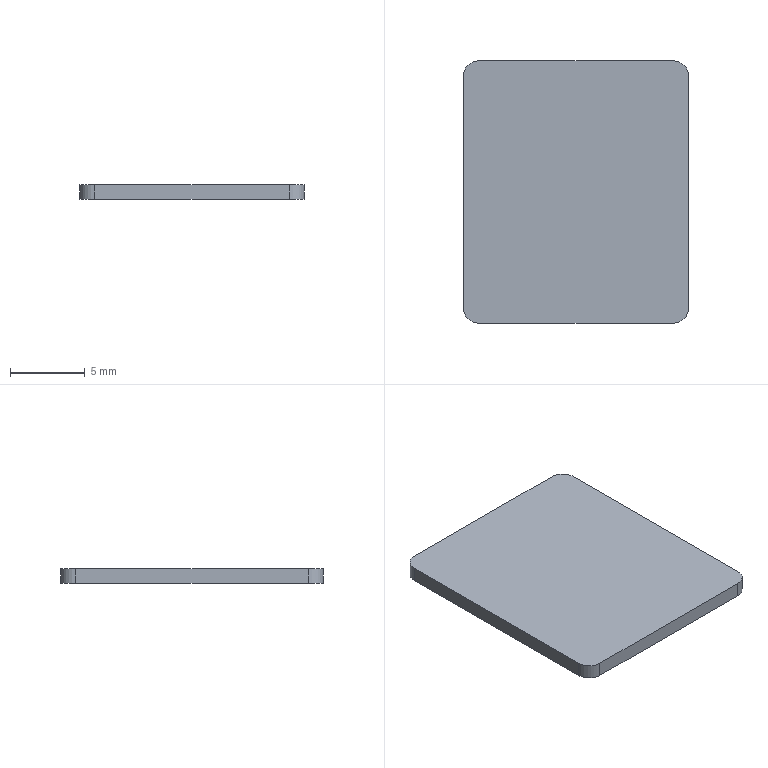Part | STEP file | 1 solid | 10 faces | box 15 x 17.5 x 1 mm | volume 261.642 mm3 | plane 6 | cylinder 4 | commonest cylinder face diameters 2 x4
STEP:
#1=CARTESIAN_POINT('',(0.,0.,0.));
#2=DIRECTION('',(0.,0.,1.));
#3=DIRECTION('',(1.,0.,0.));
#4=AXIS2_PLACEMENT_3D('',#1,#2,#3);
#5=CARTESIAN_POINT('',(6.5,6.5,38.7));
#6=VERTEX_POINT('',#5);
#7=CARTESIAN_POINT('',(-6.5,6.5,38.7));
#8=VERTEX_POINT('',#7);
#9=CARTESIAN_POINT('',(-6.5,6.5,38.7));
#10=DIRECTION('',(-1.,0.,0.));
#11=VECTOR('',#10,1.);
#12=LINE('',#9,#11);
#13=CARTESIAN_POINT('',(-6.5,5.5,38.7));
#14=DIRECTION('',(0.,0.,1.));
#15=DIRECTION('',(1.,0.,0.));
#16=AXIS2_PLACEMENT_3D('',#13,#14,#15);
#17=PLANE('',#16);
#18=CARTESIAN_POINT('',(0.,1.));
#19=DIRECTION('',(-1.,0.));
#20=VECTOR('',#19,1.);
#21=LINE('',#18,#20);
#22=(GEOMETRIC_REPRESENTATION_CONTEXT(2)PARAMETRIC_REPRESENTATION_CONTEXT()REPRESENTATION_CONTEXT('',''));
#23=DEFINITIONAL_REPRESENTATION('',(#21),#22);
#24=PCURVE('',#17,#23);
#25=CARTESIAN_POINT('',(6.5,6.5,39.7));
#26=DIRECTION('',(0.,-1.,0.));
#27=DIRECTION('',(0.,0.,-1.));
#28=AXIS2_PLACEMENT_3D('',#25,#26,#27);
#29=PLANE('',#28);
#30=CARTESIAN_POINT('',(1.,-13.));
#31=DIRECTION('',(0.,-1.));
#32=VECTOR('',#31,1.);
#33=LINE('',#30,#32);
#34=(GEOMETRIC_REPRESENTATION_CONTEXT(2)PARAMETRIC_REPRESENTATION_CONTEXT()REPRESENTATION_CONTEXT('',''));
#35=DEFINITIONAL_REPRESENTATION('',(#33),#34);
#36=PCURVE('',#29,#35);
#37=SURFACE_CURVE('',#12,(#24,#36),.PCURVE_S1.);
#38=EDGE_CURVE('',#6,#8,#37,.T.);
#39=ORIENTED_EDGE('',*,*,#38,.F.);
#40=CARTESIAN_POINT('',(7.5,5.5,38.7));
#41=VERTEX_POINT('',#40);
#42=CARTESIAN_POINT('',(6.5,5.5,38.7));
#43=DIRECTION('',(0.,0.,1.));
#44=DIRECTION('',(1.,0.,0.));
#45=AXIS2_PLACEMENT_3D('',#42,#43,#44);
#46=CIRCLE('',#45,1.);
#47=CARTESIAN_POINT('',(13.,0.));
#48=DIRECTION('',(1.,0.));
#49=AXIS2_PLACEMENT_2D('',#47,#48);
#50=CIRCLE('',#49,1.);
#51=(GEOMETRIC_REPRESENTATION_CONTEXT(2)PARAMETRIC_REPRESENTATION_CONTEXT()REPRESENTATION_CONTEXT('',''));
#52=DEFINITIONAL_REPRESENTATION('',(#50),#51);
#53=PCURVE('',#17,#52);
#54=CARTESIAN_POINT('',(6.5,5.5,39.7));
#55=DIRECTION('',(0.,0.,1.));
#56=DIRECTION('',(1.,0.,0.));
#57=AXIS2_PLACEMENT_3D('',#54,#55,#56);
#58=CYLINDRICAL_SURFACE('',#57,1.);
#59=CARTESIAN_POINT('',(0.,-1.));
#60=DIRECTION('',(1.,0.));
#61=VECTOR('',#60,1.);
#62=LINE('',#59,#61);
#63=(GEOMETRIC_REPRESENTATION_CONTEXT(2)PARAMETRIC_REPRESENTATION_CONTEXT()REPRESENTATION_CONTEXT('',''));
#64=DEFINITIONAL_REPRESENTATION('',(#62),#63);
#65=PCURVE('',#58,#64);
#66=SURFACE_CURVE('',#46,(#53,#65),.PCURVE_S1.);
#67=EDGE_CURVE('',#41,#6,#66,.T.);
#68=ORIENTED_EDGE('',*,*,#67,.F.);
#69=CARTESIAN_POINT('',(7.5,-10.,38.7));
#70=VERTEX_POINT('',#69);
#71=CARTESIAN_POINT('',(7.5,5.5,38.7));
#72=DIRECTION('',(0.,1.,0.));
#73=VECTOR('',#72,1.);
#74=LINE('',#71,#73);
#75=CARTESIAN_POINT('',(14.,0.));
#76=DIRECTION('',(0.,1.));
#77=VECTOR('',#76,1.);
#78=LINE('',#75,#77);
#79=(GEOMETRIC_REPRESENTATION_CONTEXT(2)PARAMETRIC_REPRESENTATION_CONTEXT()REPRESENTATION_CONTEXT('',''));
#80=DEFINITIONAL_REPRESENTATION('',(#78),#79);
#81=PCURVE('',#17,#80);
#82=CARTESIAN_POINT('',(7.5,-10.,39.7));
#83=DIRECTION('',(-1.,0.,0.));
#84=DIRECTION('',(0.,0.,1.));
#85=AXIS2_PLACEMENT_3D('',#82,#83,#84);
#86=PLANE('',#85);
#87=CARTESIAN_POINT('',(-1.,15.5));
#88=DIRECTION('',(0.,1.));
#89=VECTOR('',#88,1.);
#90=LINE('',#87,#89);
#91=(GEOMETRIC_REPRESENTATION_CONTEXT(2)PARAMETRIC_REPRESENTATION_CONTEXT()REPRESENTATION_CONTEXT('',''));
#92=DEFINITIONAL_REPRESENTATION('',(#90),#91);
#93=PCURVE('',#86,#92);
#94=SURFACE_CURVE('',#74,(#81,#93),.PCURVE_S1.);
#95=EDGE_CURVE('',#70,#41,#94,.T.);
#96=ORIENTED_EDGE('',*,*,#95,.F.);
#97=CARTESIAN_POINT('',(6.5,-11.,38.7));
#98=VERTEX_POINT('',#97);
#99=CARTESIAN_POINT('',(6.5,-10.,38.7));
#100=DIRECTION('',(0.,0.,1.));
#101=DIRECTION('',(1.,0.,0.));
#102=AXIS2_PLACEMENT_3D('',#99,#100,#101);
#103=CIRCLE('',#102,1.);
#104=CARTESIAN_POINT('',(13.,-15.5));
#105=DIRECTION('',(1.,0.));
#106=AXIS2_PLACEMENT_2D('',#104,#105);
#107=CIRCLE('',#106,1.);
#108=(GEOMETRIC_REPRESENTATION_CONTEXT(2)PARAMETRIC_REPRESENTATION_CONTEXT()REPRESENTATION_CONTEXT('',''));
#109=DEFINITIONAL_REPRESENTATION('',(#107),#108);
#110=PCURVE('',#17,#109);
#111=CARTESIAN_POINT('',(6.5,-10.,39.7));
#112=DIRECTION('',(0.,0.,1.));
#113=DIRECTION('',(1.,0.,0.));
#114=AXIS2_PLACEMENT_3D('',#111,#112,#113);
#115=CYLINDRICAL_SURFACE('',#114,1.);
#116=CARTESIAN_POINT('',(0.,-1.));
#117=DIRECTION('',(1.,0.));
#118=VECTOR('',#117,1.);
#119=LINE('',#116,#118);
#120=(GEOMETRIC_REPRESENTATION_CONTEXT(2)PARAMETRIC_REPRESENTATION_CONTEXT()REPRESENTATION_CONTEXT('',''));
#121=DEFINITIONAL_REPRESENTATION('',(#119),#120);
#122=PCURVE('',#115,#121);
#123=SURFACE_CURVE('',#103,(#110,#122),.PCURVE_S1.);
#124=EDGE_CURVE('',#98,#70,#123,.T.);
#125=ORIENTED_EDGE('',*,*,#124,.F.);
#126=CARTESIAN_POINT('',(-6.5,-11.,38.7));
#127=VERTEX_POINT('',#126);
#128=CARTESIAN_POINT('',(-6.5,-11.,38.7));
#129=DIRECTION('',(1.,0.,0.));
#130=VECTOR('',#129,1.);
#131=LINE('',#128,#130);
#132=CARTESIAN_POINT('',(0.,-16.5));
#133=DIRECTION('',(1.,0.));
#134=VECTOR('',#133,1.);
#135=LINE('',#132,#134);
#136=(GEOMETRIC_REPRESENTATION_CONTEXT(2)PARAMETRIC_REPRESENTATION_CONTEXT()REPRESENTATION_CONTEXT('',''));
#137=DEFINITIONAL_REPRESENTATION('',(#135),#136);
#138=PCURVE('',#17,#137);
#139=CARTESIAN_POINT('',(-6.5,-11.,39.7));
#140=DIRECTION('',(0.,1.,0.));
#141=DIRECTION('',(1.,0.,0.));
#142=AXIS2_PLACEMENT_3D('',#139,#140,#141);
#143=PLANE('',#142);
#144=CARTESIAN_POINT('',(0.,1.));
#145=DIRECTION('',(1.,0.));
#146=VECTOR('',#145,1.);
#147=LINE('',#144,#146);
#148=(GEOMETRIC_REPRESENTATION_CONTEXT(2)PARAMETRIC_REPRESENTATION_CONTEXT()REPRESENTATION_CONTEXT('',''));
#149=DEFINITIONAL_REPRESENTATION('',(#147),#148);
#150=PCURVE('',#143,#149);
#151=SURFACE_CURVE('',#131,(#138,#150),.PCURVE_S1.);
#152=EDGE_CURVE('',#127,#98,#151,.T.);
#153=ORIENTED_EDGE('',*,*,#152,.F.);
#154=CARTESIAN_POINT('',(-7.5,-10.,38.7));
#155=VERTEX_POINT('',#154);
#156=CARTESIAN_POINT('',(-6.5,-10.,38.7));
#157=DIRECTION('',(0.,0.,1.));
#158=DIRECTION('',(1.,0.,0.));
#159=AXIS2_PLACEMENT_3D('',#156,#157,#158);
#160=CIRCLE('',#159,1.);
#161=CARTESIAN_POINT('',(0.,-15.5));
#162=DIRECTION('',(1.,0.));
#163=AXIS2_PLACEMENT_2D('',#161,#162);
#164=CIRCLE('',#163,1.);
#165=(GEOMETRIC_REPRESENTATION_CONTEXT(2)PARAMETRIC_REPRESENTATION_CONTEXT()REPRESENTATION_CONTEXT('',''));
#166=DEFINITIONAL_REPRESENTATION('',(#164),#165);
#167=PCURVE('',#17,#166);
#168=CARTESIAN_POINT('',(-6.5,-10.,39.7));
#169=DIRECTION('',(0.,0.,1.));
#170=DIRECTION('',(1.,0.,0.));
#171=AXIS2_PLACEMENT_3D('',#168,#169,#170);
#172=CYLINDRICAL_SURFACE('',#171,1.);
#173=CARTESIAN_POINT('',(0.,-1.));
#174=DIRECTION('',(1.,0.));
#175=VECTOR('',#174,1.);
#176=LINE('',#173,#175);
#177=(GEOMETRIC_REPRESENTATION_CONTEXT(2)PARAMETRIC_REPRESENTATION_CONTEXT()REPRESENTATION_CONTEXT('',''));
#178=DEFINITIONAL_REPRESENTATION('',(#176),#177);
#179=PCURVE('',#172,#178);
#180=SURFACE_CURVE('',#160,(#167,#179),.PCURVE_S1.);
#181=EDGE_CURVE('',#155,#127,#180,.T.);
#182=ORIENTED_EDGE('',*,*,#181,.F.);
#183=CARTESIAN_POINT('',(-7.5,5.5,38.7));
#184=VERTEX_POINT('',#183);
#185=CARTESIAN_POINT('',(-7.5,5.5,38.7));
#186=DIRECTION('',(0.,-1.,0.));
#187=VECTOR('',#186,1.);
#188=LINE('',#185,#187);
#189=CARTESIAN_POINT('',(-1.,0.));
#190=DIRECTION('',(0.,-1.));
#191=VECTOR('',#190,1.);
#192=LINE('',#189,#191);
#193=(GEOMETRIC_REPRESENTATION_CONTEXT(2)PARAMETRIC_REPRESENTATION_CONTEXT()REPRESENTATION_CONTEXT('',''));
#194=DEFINITIONAL_REPRESENTATION('',(#192),#193);
#195=PCURVE('',#17,#194);
#196=CARTESIAN_POINT('',(-7.5,5.5,39.7));
#197=DIRECTION('',(1.,0.,0.));
#198=DIRECTION('',(0.,1.,0.));
#199=AXIS2_PLACEMENT_3D('',#196,#197,#198);
#200=PLANE('',#199);
#201=CARTESIAN_POINT('',(0.,-1.));
#202=DIRECTION('',(-1.,0.));
#203=VECTOR('',#202,1.);
#204=LINE('',#201,#203);
#205=(GEOMETRIC_REPRESENTATION_CONTEXT(2)PARAMETRIC_REPRESENTATION_CONTEXT()REPRESENTATION_CONTEXT('',''));
#206=DEFINITIONAL_REPRESENTATION('',(#204),#205);
#207=PCURVE('',#200,#206);
#208=SURFACE_CURVE('',#188,(#195,#207),.PCURVE_S1.);
#209=EDGE_CURVE('',#184,#155,#208,.T.);
#210=ORIENTED_EDGE('',*,*,#209,.F.);
#211=CARTESIAN_POINT('',(-6.5,5.5,38.7));
#212=DIRECTION('',(0.,0.,1.));
#213=DIRECTION('',(1.,0.,0.));
#214=AXIS2_PLACEMENT_3D('',#211,#212,#213);
#215=CIRCLE('',#214,1.);
#216=CARTESIAN_POINT('',(0.,0.));
#217=DIRECTION('',(1.,0.));
#218=AXIS2_PLACEMENT_2D('',#216,#217);
#219=CIRCLE('',#218,1.);
#220=(GEOMETRIC_REPRESENTATION_CONTEXT(2)PARAMETRIC_REPRESENTATION_CONTEXT()REPRESENTATION_CONTEXT('',''));
#221=DEFINITIONAL_REPRESENTATION('',(#219),#220);
#222=PCURVE('',#17,#221);
#223=CARTESIAN_POINT('',(-6.5,5.5,39.7));
#224=DIRECTION('',(0.,0.,1.));
#225=DIRECTION('',(1.,0.,0.));
#226=AXIS2_PLACEMENT_3D('',#223,#224,#225);
#227=CYLINDRICAL_SURFACE('',#226,1.);
#228=CARTESIAN_POINT('',(0.,-1.));
#229=DIRECTION('',(1.,0.));
#230=VECTOR('',#229,1.);
#231=LINE('',#228,#230);
#232=(GEOMETRIC_REPRESENTATION_CONTEXT(2)PARAMETRIC_REPRESENTATION_CONTEXT()REPRESENTATION_CONTEXT('',''));
#233=DEFINITIONAL_REPRESENTATION('',(#231),#232);
#234=PCURVE('',#227,#233);
#235=SURFACE_CURVE('',#215,(#222,#234),.PCURVE_S1.);
#236=EDGE_CURVE('',#8,#184,#235,.T.);
#237=ORIENTED_EDGE('',*,*,#236,.F.);
#238=EDGE_LOOP('',(#39,#68,#96,#125,#153,#182,#210,#237));
#239=FACE_BOUND('',#238,.T.);
#240=ADVANCED_FACE('',(#239),#17,.F.);
#241=CARTESIAN_POINT('',(-6.5,6.5,39.7));
#242=VERTEX_POINT('',#241);
#243=CARTESIAN_POINT('',(-7.5,5.5,39.7));
#244=VERTEX_POINT('',#243);
#245=CARTESIAN_POINT('',(-6.5,5.5,39.7));
#246=DIRECTION('',(0.,0.,1.));
#247=DIRECTION('',(1.,0.,0.));
#248=AXIS2_PLACEMENT_3D('',#245,#246,#247);
#249=CIRCLE('',#248,1.);
#250=CARTESIAN_POINT('',(0.,0.));
#251=DIRECTION('',(1.,0.));
#252=VECTOR('',#251,1.);
#253=LINE('',#250,#252);
#254=(GEOMETRIC_REPRESENTATION_CONTEXT(2)PARAMETRIC_REPRESENTATION_CONTEXT()REPRESENTATION_CONTEXT('',''));
#255=DEFINITIONAL_REPRESENTATION('',(#253),#254);
#256=PCURVE('',#227,#255);
#257=CARTESIAN_POINT('',(-6.5,5.5,39.7));
#258=DIRECTION('',(0.,0.,1.));
#259=DIRECTION('',(1.,0.,0.));
#260=AXIS2_PLACEMENT_3D('',#257,#258,#259);
#261=PLANE('',#260);
#262=CARTESIAN_POINT('',(0.,0.));
#263=DIRECTION('',(1.,0.));
#264=AXIS2_PLACEMENT_2D('',#262,#263);
#265=CIRCLE('',#264,1.);
#266=(GEOMETRIC_REPRESENTATION_CONTEXT(2)PARAMETRIC_REPRESENTATION_CONTEXT()REPRESENTATION_CONTEXT('',''));
#267=DEFINITIONAL_REPRESENTATION('',(#265),#266);
#268=PCURVE('',#261,#267);
#269=SURFACE_CURVE('',#249,(#256,#268),.PCURVE_S1.);
#270=EDGE_CURVE('',#242,#244,#269,.T.);
#271=ORIENTED_EDGE('',*,*,#270,.F.);
#272=CARTESIAN_POINT('',(-6.5,6.5,39.7));
#273=DIRECTION('',(0.,0.,-1.));
#274=VECTOR('',#273,1.);
#275=LINE('',#272,#274);
#276=CARTESIAN_POINT('',(1.571,0.));
#277=DIRECTION('',(0.,-1.));
#278=VECTOR('',#277,1.);
#279=LINE('',#276,#278);
#280=(GEOMETRIC_REPRESENTATION_CONTEXT(2)PARAMETRIC_REPRESENTATION_CONTEXT()REPRESENTATION_CONTEXT('',''));
#281=DEFINITIONAL_REPRESENTATION('',(#279),#280);
#282=PCURVE('',#227,#281);
#283=CARTESIAN_POINT('',(0.,-13.));
#284=DIRECTION('',(1.,0.));
#285=VECTOR('',#284,1.);
#286=LINE('',#283,#285);
#287=(GEOMETRIC_REPRESENTATION_CONTEXT(2)PARAMETRIC_REPRESENTATION_CONTEXT()REPRESENTATION_CONTEXT('',''));
#288=DEFINITIONAL_REPRESENTATION('',(#286),#287);
#289=PCURVE('',#29,#288);
#290=SURFACE_CURVE('',#275,(#282,#289),.PCURVE_S1.);
#291=EDGE_CURVE('',#242,#8,#290,.T.);
#292=ORIENTED_EDGE('',*,*,#291,.T.);
#293=ORIENTED_EDGE('',*,*,#236,.T.);
#294=CARTESIAN_POINT('',(-7.5,5.5,39.7));
#295=DIRECTION('',(0.,0.,1.));
#296=VECTOR('',#295,1.);
#297=LINE('',#294,#296);
#298=CARTESIAN_POINT('',(3.142,0.));
#299=DIRECTION('',(0.,1.));
#300=VECTOR('',#299,1.);
#301=LINE('',#298,#300);
#302=(GEOMETRIC_REPRESENTATION_CONTEXT(2)PARAMETRIC_REPRESENTATION_CONTEXT()REPRESENTATION_CONTEXT('',''));
#303=DEFINITIONAL_REPRESENTATION('',(#301),#302);
#304=PCURVE('',#227,#303);
#305=CARTESIAN_POINT('',(0.,0.));
#306=DIRECTION('',(0.,1.));
#307=VECTOR('',#306,1.);
#308=LINE('',#305,#307);
#309=(GEOMETRIC_REPRESENTATION_CONTEXT(2)PARAMETRIC_REPRESENTATION_CONTEXT()REPRESENTATION_CONTEXT('',''));
#310=DEFINITIONAL_REPRESENTATION('',(#308),#309);
#311=PCURVE('',#200,#310);
#312=SURFACE_CURVE('',#297,(#304,#311),.PCURVE_S1.);
#313=EDGE_CURVE('',#184,#244,#312,.T.);
#314=ORIENTED_EDGE('',*,*,#313,.T.);
#315=EDGE_LOOP('',(#271,#292,#293,#314));
#316=FACE_BOUND('',#315,.T.);
#317=ADVANCED_FACE('',(#316),#227,.T.);
#318=ORIENTED_EDGE('',*,*,#291,.F.);
#319=CARTESIAN_POINT('',(6.5,6.5,39.7));
#320=VERTEX_POINT('',#319);
#321=CARTESIAN_POINT('',(6.5,6.5,39.7));
#322=DIRECTION('',(-1.,0.,0.));
#323=VECTOR('',#322,1.);
#324=LINE('',#321,#323);
#325=CARTESIAN_POINT('',(0.,0.));
#326=DIRECTION('',(0.,-1.));
#327=VECTOR('',#326,1.);
#328=LINE('',#325,#327);
#329=(GEOMETRIC_REPRESENTATION_CONTEXT(2)PARAMETRIC_REPRESENTATION_CONTEXT()REPRESENTATION_CONTEXT('',''));
#330=DEFINITIONAL_REPRESENTATION('',(#328),#329);
#331=PCURVE('',#29,#330);
#332=CARTESIAN_POINT('',(13.,1.));
#333=DIRECTION('',(-1.,0.));
#334=VECTOR('',#333,1.);
#335=LINE('',#332,#334);
#336=(GEOMETRIC_REPRESENTATION_CONTEXT(2)PARAMETRIC_REPRESENTATION_CONTEXT()REPRESENTATION_CONTEXT('',''));
#337=DEFINITIONAL_REPRESENTATION('',(#335),#336);
#338=PCURVE('',#261,#337);
#339=SURFACE_CURVE('',#324,(#331,#338),.PCURVE_S1.);
#340=EDGE_CURVE('',#320,#242,#339,.T.);
#341=ORIENTED_EDGE('',*,*,#340,.F.);
#342=CARTESIAN_POINT('',(6.5,6.5,39.7));
#343=DIRECTION('',(0.,0.,1.));
#344=VECTOR('',#343,1.);
#345=LINE('',#342,#344);
#346=CARTESIAN_POINT('',(0.,0.));
#347=DIRECTION('',(-1.,0.));
#348=VECTOR('',#347,1.);
#349=LINE('',#346,#348);
#350=(GEOMETRIC_REPRESENTATION_CONTEXT(2)PARAMETRIC_REPRESENTATION_CONTEXT()REPRESENTATION_CONTEXT('',''));
#351=DEFINITIONAL_REPRESENTATION('',(#349),#350);
#352=PCURVE('',#29,#351);
#353=CARTESIAN_POINT('',(1.571,0.));
#354=DIRECTION('',(0.,1.));
#355=VECTOR('',#354,1.);
#356=LINE('',#353,#355);
#357=(GEOMETRIC_REPRESENTATION_CONTEXT(2)PARAMETRIC_REPRESENTATION_CONTEXT()REPRESENTATION_CONTEXT('',''));
#358=DEFINITIONAL_REPRESENTATION('',(#356),#357);
#359=PCURVE('',#58,#358);
#360=SURFACE_CURVE('',#345,(#352,#359),.PCURVE_S1.);
#361=EDGE_CURVE('',#6,#320,#360,.T.);
#362=ORIENTED_EDGE('',*,*,#361,.F.);
#363=ORIENTED_EDGE('',*,*,#38,.T.);
#364=EDGE_LOOP('',(#318,#341,#362,#363));
#365=FACE_BOUND('',#364,.T.);
#366=ADVANCED_FACE('',(#365),#29,.F.);
#367=CARTESIAN_POINT('',(7.5,5.5,39.7));
#368=VERTEX_POINT('',#367);
#369=CARTESIAN_POINT('',(6.5,5.5,39.7));
#370=DIRECTION('',(0.,0.,-1.));
#371=DIRECTION('',(1.,0.,0.));
#372=AXIS2_PLACEMENT_3D('',#369,#370,#371);
#373=CIRCLE('',#372,1.);
#374=CARTESIAN_POINT('',(6.283,0.));
#375=DIRECTION('',(-1.,0.));
#376=VECTOR('',#375,1.);
#377=LINE('',#374,#376);
#378=(GEOMETRIC_REPRESENTATION_CONTEXT(2)PARAMETRIC_REPRESENTATION_CONTEXT()REPRESENTATION_CONTEXT('',''));
#379=DEFINITIONAL_REPRESENTATION('',(#377),#378);
#380=PCURVE('',#58,#379);
#381=CARTESIAN_POINT('',(14.,0.));
#382=CARTESIAN_POINT('',(14.,-1.732));
#383=CARTESIAN_POINT('',(12.5,-0.866));
#384=CARTESIAN_POINT('',(11.,0.));
#385=CARTESIAN_POINT('',(12.5,0.866));
#386=CARTESIAN_POINT('',(14.,1.732));
#387=CARTESIAN_POINT('',(14.,0.));
#388=(BOUNDED_CURVE()B_SPLINE_CURVE(2,(#381,#382,#383,#384,#385,#386,#387),.UNSPECIFIED.,.T.,.F.)B_SPLINE_CURVE_WITH_KNOTS((1,2,2,2,2,1),(-2.094,0.,2.094,4.189,6.283,8.378),.UNSPECIFIED.)CURVE()GEOMETRIC_REPRESENTATION_ITEM()RATIONAL_B_SPLINE_CURVE((1.,0.5,1.,0.5,1.,0.5,1.))REPRESENTATION_ITEM(''));
#389=(GEOMETRIC_REPRESENTATION_CONTEXT(2)PARAMETRIC_REPRESENTATION_CONTEXT()REPRESENTATION_CONTEXT('',''));
#390=DEFINITIONAL_REPRESENTATION('',(#388),#389);
#391=PCURVE('',#261,#390);
#392=SURFACE_CURVE('',#373,(#380,#391),.PCURVE_S1.);
#393=EDGE_CURVE('',#320,#368,#392,.T.);
#394=ORIENTED_EDGE('',*,*,#393,.T.);
#395=CARTESIAN_POINT('',(7.5,5.5,39.7));
#396=DIRECTION('',(0.,0.,-1.));
#397=VECTOR('',#396,1.);
#398=LINE('',#395,#397);
#399=CARTESIAN_POINT('',(0.,0.));
#400=DIRECTION('',(0.,-1.));
#401=VECTOR('',#400,1.);
#402=LINE('',#399,#401);
#403=(GEOMETRIC_REPRESENTATION_CONTEXT(2)PARAMETRIC_REPRESENTATION_CONTEXT()REPRESENTATION_CONTEXT('',''));
#404=DEFINITIONAL_REPRESENTATION('',(#402),#403);
#405=PCURVE('',#58,#404);
#406=CARTESIAN_POINT('',(0.,15.5));
#407=DIRECTION('',(-1.,0.));
#408=VECTOR('',#407,1.);
#409=LINE('',#406,#408);
#410=(GEOMETRIC_REPRESENTATION_CONTEXT(2)PARAMETRIC_REPRESENTATION_CONTEXT()REPRESENTATION_CONTEXT('',''));
#411=DEFINITIONAL_REPRESENTATION('',(#409),#410);
#412=PCURVE('',#86,#411);
#413=SURFACE_CURVE('',#398,(#405,#412),.PCURVE_S1.);
#414=EDGE_CURVE('',#368,#41,#413,.T.);
#415=ORIENTED_EDGE('',*,*,#414,.T.);
#416=ORIENTED_EDGE('',*,*,#67,.T.);
#417=ORIENTED_EDGE('',*,*,#361,.T.);
#418=EDGE_LOOP('',(#394,#415,#416,#417));
#419=FACE_BOUND('',#418,.T.);
#420=ADVANCED_FACE('',(#419),#58,.T.);
#421=ORIENTED_EDGE('',*,*,#414,.F.);
#422=CARTESIAN_POINT('',(7.5,-10.,39.7));
#423=VERTEX_POINT('',#422);
#424=CARTESIAN_POINT('',(7.5,-10.,39.7));
#425=DIRECTION('',(0.,1.,0.));
#426=VECTOR('',#425,1.);
#427=LINE('',#424,#426);
#428=CARTESIAN_POINT('',(0.,0.));
#429=DIRECTION('',(0.,1.));
#430=VECTOR('',#429,1.);
#431=LINE('',#428,#430);
#432=(GEOMETRIC_REPRESENTATION_CONTEXT(2)PARAMETRIC_REPRESENTATION_CONTEXT()REPRESENTATION_CONTEXT('',''));
#433=DEFINITIONAL_REPRESENTATION('',(#431),#432);
#434=PCURVE('',#86,#433);
#435=CARTESIAN_POINT('',(14.,-15.5));
#436=DIRECTION('',(0.,1.));
#437=VECTOR('',#436,1.);
#438=LINE('',#435,#437);
#439=(GEOMETRIC_REPRESENTATION_CONTEXT(2)PARAMETRIC_REPRESENTATION_CONTEXT()REPRESENTATION_CONTEXT('',''));
#440=DEFINITIONAL_REPRESENTATION('',(#438),#439);
#441=PCURVE('',#261,#440);
#442=SURFACE_CURVE('',#427,(#434,#441),.PCURVE_S1.);
#443=EDGE_CURVE('',#423,#368,#442,.T.);
#444=ORIENTED_EDGE('',*,*,#443,.F.);
#445=CARTESIAN_POINT('',(7.5,-10.,39.7));
#446=DIRECTION('',(0.,0.,1.));
#447=VECTOR('',#446,1.);
#448=LINE('',#445,#447);
#449=CARTESIAN_POINT('',(0.,0.));
#450=DIRECTION('',(1.,0.));
#451=VECTOR('',#450,1.);
#452=LINE('',#449,#451);
#453=(GEOMETRIC_REPRESENTATION_CONTEXT(2)PARAMETRIC_REPRESENTATION_CONTEXT()REPRESENTATION_CONTEXT('',''));
#454=DEFINITIONAL_REPRESENTATION('',(#452),#453);
#455=PCURVE('',#86,#454);
#456=CARTESIAN_POINT('',(6.283,0.));
#457=DIRECTION('',(0.,1.));
#458=VECTOR('',#457,1.);
#459=LINE('',#456,#458);
#460=(GEOMETRIC_REPRESENTATION_CONTEXT(2)PARAMETRIC_REPRESENTATION_CONTEXT()REPRESENTATION_CONTEXT('',''));
#461=DEFINITIONAL_REPRESENTATION('',(#459),#460);
#462=PCURVE('',#115,#461);
#463=SURFACE_CURVE('',#448,(#455,#462),.PCURVE_S1.);
#464=EDGE_CURVE('',#70,#423,#463,.T.);
#465=ORIENTED_EDGE('',*,*,#464,.F.);
#466=ORIENTED_EDGE('',*,*,#95,.T.);
#467=EDGE_LOOP('',(#421,#444,#465,#466));
#468=FACE_BOUND('',#467,.T.);
#469=ADVANCED_FACE('',(#468),#86,.F.);
#470=CARTESIAN_POINT('',(6.5,-11.,39.7));
#471=VERTEX_POINT('',#470);
#472=CARTESIAN_POINT('',(6.5,-10.,39.7));
#473=DIRECTION('',(0.,0.,-1.));
#474=DIRECTION('',(1.,0.,0.));
#475=AXIS2_PLACEMENT_3D('',#472,#473,#474);
#476=CIRCLE('',#475,1.);
#477=CARTESIAN_POINT('',(6.283,0.));
#478=DIRECTION('',(-1.,0.));
#479=VECTOR('',#478,1.);
#480=LINE('',#477,#479);
#481=(GEOMETRIC_REPRESENTATION_CONTEXT(2)PARAMETRIC_REPRESENTATION_CONTEXT()REPRESENTATION_CONTEXT('',''));
#482=DEFINITIONAL_REPRESENTATION('',(#480),#481);
#483=PCURVE('',#115,#482);
#484=CARTESIAN_POINT('',(14.,-15.5));
#485=CARTESIAN_POINT('',(14.,-17.232));
#486=CARTESIAN_POINT('',(12.5,-16.366));
#487=CARTESIAN_POINT('',(11.,-15.5));
#488=CARTESIAN_POINT('',(12.5,-14.634));
#489=CARTESIAN_POINT('',(14.,-13.768));
#490=CARTESIAN_POINT('',(14.,-15.5));
#491=(BOUNDED_CURVE()B_SPLINE_CURVE(2,(#484,#485,#486,#487,#488,#489,#490),.UNSPECIFIED.,.T.,.F.)B_SPLINE_CURVE_WITH_KNOTS((1,2,2,2,2,1),(-2.094,0.,2.094,4.189,6.283,8.378),.UNSPECIFIED.)CURVE()GEOMETRIC_REPRESENTATION_ITEM()RATIONAL_B_SPLINE_CURVE((1.,0.5,1.,0.5,1.,0.5,1.))REPRESENTATION_ITEM(''));
#492=(GEOMETRIC_REPRESENTATION_CONTEXT(2)PARAMETRIC_REPRESENTATION_CONTEXT()REPRESENTATION_CONTEXT('',''));
#493=DEFINITIONAL_REPRESENTATION('',(#491),#492);
#494=PCURVE('',#261,#493);
#495=SURFACE_CURVE('',#476,(#483,#494),.PCURVE_S1.);
#496=EDGE_CURVE('',#423,#471,#495,.T.);
#497=ORIENTED_EDGE('',*,*,#496,.T.);
#498=CARTESIAN_POINT('',(6.5,-11.,39.7));
#499=DIRECTION('',(0.,0.,-1.));
#500=VECTOR('',#499,1.);
#501=LINE('',#498,#500);
#502=CARTESIAN_POINT('',(4.712,0.));
#503=DIRECTION('',(0.,-1.));
#504=VECTOR('',#503,1.);
#505=LINE('',#502,#504);
#506=(GEOMETRIC_REPRESENTATION_CONTEXT(2)PARAMETRIC_REPRESENTATION_CONTEXT()REPRESENTATION_CONTEXT('',''));
#507=DEFINITIONAL_REPRESENTATION('',(#505),#506);
#508=PCURVE('',#115,#507);
#509=CARTESIAN_POINT('',(13.,0.));
#510=DIRECTION('',(0.,1.));
#511=VECTOR('',#510,1.);
#512=LINE('',#509,#511);
#513=(GEOMETRIC_REPRESENTATION_CONTEXT(2)PARAMETRIC_REPRESENTATION_CONTEXT()REPRESENTATION_CONTEXT('',''));
#514=DEFINITIONAL_REPRESENTATION('',(#512),#513);
#515=PCURVE('',#143,#514);
#516=SURFACE_CURVE('',#501,(#508,#515),.PCURVE_S1.);
#517=EDGE_CURVE('',#471,#98,#516,.T.);
#518=ORIENTED_EDGE('',*,*,#517,.T.);
#519=ORIENTED_EDGE('',*,*,#124,.T.);
#520=ORIENTED_EDGE('',*,*,#464,.T.);
#521=EDGE_LOOP('',(#497,#518,#519,#520));
#522=FACE_BOUND('',#521,.T.);
#523=ADVANCED_FACE('',(#522),#115,.T.);
#524=ORIENTED_EDGE('',*,*,#517,.F.);
#525=CARTESIAN_POINT('',(-6.5,-11.,39.7));
#526=VERTEX_POINT('',#525);
#527=CARTESIAN_POINT('',(-6.5,-11.,39.7));
#528=DIRECTION('',(1.,0.,0.));
#529=VECTOR('',#528,1.);
#530=LINE('',#527,#529);
#531=CARTESIAN_POINT('',(0.,0.));
#532=DIRECTION('',(1.,0.));
#533=VECTOR('',#532,1.);
#534=LINE('',#531,#533);
#535=(GEOMETRIC_REPRESENTATION_CONTEXT(2)PARAMETRIC_REPRESENTATION_CONTEXT()REPRESENTATION_CONTEXT('',''));
#536=DEFINITIONAL_REPRESENTATION('',(#534),#535);
#537=PCURVE('',#143,#536);
#538=CARTESIAN_POINT('',(0.,-16.5));
#539=DIRECTION('',(1.,0.));
#540=VECTOR('',#539,1.);
#541=LINE('',#538,#540);
#542=(GEOMETRIC_REPRESENTATION_CONTEXT(2)PARAMETRIC_REPRESENTATION_CONTEXT()REPRESENTATION_CONTEXT('',''));
#543=DEFINITIONAL_REPRESENTATION('',(#541),#542);
#544=PCURVE('',#261,#543);
#545=SURFACE_CURVE('',#530,(#537,#544),.PCURVE_S1.);
#546=EDGE_CURVE('',#526,#471,#545,.T.);
#547=ORIENTED_EDGE('',*,*,#546,.F.);
#548=CARTESIAN_POINT('',(-6.5,-11.,39.7));
#549=DIRECTION('',(0.,0.,1.));
#550=VECTOR('',#549,1.);
#551=LINE('',#548,#550);
#552=CARTESIAN_POINT('',(0.,0.));
#553=DIRECTION('',(0.,-1.));
#554=VECTOR('',#553,1.);
#555=LINE('',#552,#554);
#556=(GEOMETRIC_REPRESENTATION_CONTEXT(2)PARAMETRIC_REPRESENTATION_CONTEXT()REPRESENTATION_CONTEXT('',''));
#557=DEFINITIONAL_REPRESENTATION('',(#555),#556);
#558=PCURVE('',#143,#557);
#559=CARTESIAN_POINT('',(4.712,0.));
#560=DIRECTION('',(0.,1.));
#561=VECTOR('',#560,1.);
#562=LINE('',#559,#561);
#563=(GEOMETRIC_REPRESENTATION_CONTEXT(2)PARAMETRIC_REPRESENTATION_CONTEXT()REPRESENTATION_CONTEXT('',''));
#564=DEFINITIONAL_REPRESENTATION('',(#562),#563);
#565=PCURVE('',#172,#564);
#566=SURFACE_CURVE('',#551,(#558,#565),.PCURVE_S1.);
#567=EDGE_CURVE('',#127,#526,#566,.T.);
#568=ORIENTED_EDGE('',*,*,#567,.F.);
#569=ORIENTED_EDGE('',*,*,#152,.T.);
#570=EDGE_LOOP('',(#524,#547,#568,#569));
#571=FACE_BOUND('',#570,.T.);
#572=ADVANCED_FACE('',(#571),#143,.F.);
#573=CARTESIAN_POINT('',(-7.5,-10.,39.7));
#574=VERTEX_POINT('',#573);
#575=CARTESIAN_POINT('',(-6.5,-10.,39.7));
#576=DIRECTION('',(0.,0.,-1.));
#577=DIRECTION('',(1.,0.,0.));
#578=AXIS2_PLACEMENT_3D('',#575,#576,#577);
#579=CIRCLE('',#578,1.);
#580=CARTESIAN_POINT('',(6.283,0.));
#581=DIRECTION('',(-1.,0.));
#582=VECTOR('',#581,1.);
#583=LINE('',#580,#582);
#584=(GEOMETRIC_REPRESENTATION_CONTEXT(2)PARAMETRIC_REPRESENTATION_CONTEXT()REPRESENTATION_CONTEXT('',''));
#585=DEFINITIONAL_REPRESENTATION('',(#583),#584);
#586=PCURVE('',#172,#585);
#587=CARTESIAN_POINT('',(1.,-15.5));
#588=CARTESIAN_POINT('',(1.,-17.232));
#589=CARTESIAN_POINT('',(-0.5,-16.366));
#590=CARTESIAN_POINT('',(-2.,-15.5));
#591=CARTESIAN_POINT('',(-0.5,-14.634));
#592=CARTESIAN_POINT('',(1.,-13.768));
#593=CARTESIAN_POINT('',(1.,-15.5));
#594=(BOUNDED_CURVE()B_SPLINE_CURVE(2,(#587,#588,#589,#590,#591,#592,#593),.UNSPECIFIED.,.T.,.F.)B_SPLINE_CURVE_WITH_KNOTS((1,2,2,2,2,1),(-2.094,0.,2.094,4.189,6.283,8.378),.UNSPECIFIED.)CURVE()GEOMETRIC_REPRESENTATION_ITEM()RATIONAL_B_SPLINE_CURVE((1.,0.5,1.,0.5,1.,0.5,1.))REPRESENTATION_ITEM(''));
#595=(GEOMETRIC_REPRESENTATION_CONTEXT(2)PARAMETRIC_REPRESENTATION_CONTEXT()REPRESENTATION_CONTEXT('',''));
#596=DEFINITIONAL_REPRESENTATION('',(#594),#595);
#597=PCURVE('',#261,#596);
#598=SURFACE_CURVE('',#579,(#586,#597),.PCURVE_S1.);
#599=EDGE_CURVE('',#526,#574,#598,.T.);
#600=ORIENTED_EDGE('',*,*,#599,.T.);
#601=CARTESIAN_POINT('',(-7.5,-10.,39.7));
#602=DIRECTION('',(0.,0.,-1.));
#603=VECTOR('',#602,1.);
#604=LINE('',#601,#603);
#605=CARTESIAN_POINT('',(3.142,0.));
#606=DIRECTION('',(0.,-1.));
#607=VECTOR('',#606,1.);
#608=LINE('',#605,#607);
#609=(GEOMETRIC_REPRESENTATION_CONTEXT(2)PARAMETRIC_REPRESENTATION_CONTEXT()REPRESENTATION_CONTEXT('',''));
#610=DEFINITIONAL_REPRESENTATION('',(#608),#609);
#611=PCURVE('',#172,#610);
#612=CARTESIAN_POINT('',(-15.5,0.));
#613=DIRECTION('',(0.,-1.));
#614=VECTOR('',#613,1.);
#615=LINE('',#612,#614);
#616=(GEOMETRIC_REPRESENTATION_CONTEXT(2)PARAMETRIC_REPRESENTATION_CONTEXT()REPRESENTATION_CONTEXT('',''));
#617=DEFINITIONAL_REPRESENTATION('',(#615),#616);
#618=PCURVE('',#200,#617);
#619=SURFACE_CURVE('',#604,(#611,#618),.PCURVE_S1.);
#620=EDGE_CURVE('',#574,#155,#619,.T.);
#621=ORIENTED_EDGE('',*,*,#620,.T.);
#622=ORIENTED_EDGE('',*,*,#181,.T.);
#623=ORIENTED_EDGE('',*,*,#567,.T.);
#624=EDGE_LOOP('',(#600,#621,#622,#623));
#625=FACE_BOUND('',#624,.T.);
#626=ADVANCED_FACE('',(#625),#172,.T.);
#627=ORIENTED_EDGE('',*,*,#620,.F.);
#628=CARTESIAN_POINT('',(-7.5,5.5,39.7));
#629=DIRECTION('',(0.,-1.,0.));
#630=VECTOR('',#629,1.);
#631=LINE('',#628,#630);
#632=CARTESIAN_POINT('',(0.,0.));
#633=DIRECTION('',(-1.,0.));
#634=VECTOR('',#633,1.);
#635=LINE('',#632,#634);
#636=(GEOMETRIC_REPRESENTATION_CONTEXT(2)PARAMETRIC_REPRESENTATION_CONTEXT()REPRESENTATION_CONTEXT('',''));
#637=DEFINITIONAL_REPRESENTATION('',(#635),#636);
#638=PCURVE('',#200,#637);
#639=CARTESIAN_POINT('',(-1.,0.));
#640=DIRECTION('',(0.,-1.));
#641=VECTOR('',#640,1.);
#642=LINE('',#639,#641);
#643=(GEOMETRIC_REPRESENTATION_CONTEXT(2)PARAMETRIC_REPRESENTATION_CONTEXT()REPRESENTATION_CONTEXT('',''));
#644=DEFINITIONAL_REPRESENTATION('',(#642),#643);
#645=PCURVE('',#261,#644);
#646=SURFACE_CURVE('',#631,(#638,#645),.PCURVE_S1.);
#647=EDGE_CURVE('',#244,#574,#646,.T.);
#648=ORIENTED_EDGE('',*,*,#647,.F.);
#649=ORIENTED_EDGE('',*,*,#313,.F.);
#650=ORIENTED_EDGE('',*,*,#209,.T.);
#651=EDGE_LOOP('',(#627,#648,#649,#650));
#652=FACE_BOUND('',#651,.T.);
#653=ADVANCED_FACE('',(#652),#200,.F.);
#654=ORIENTED_EDGE('',*,*,#393,.F.);
#655=ORIENTED_EDGE('',*,*,#340,.T.);
#656=ORIENTED_EDGE('',*,*,#270,.T.);
#657=ORIENTED_EDGE('',*,*,#647,.T.);
#658=ORIENTED_EDGE('',*,*,#599,.F.);
#659=ORIENTED_EDGE('',*,*,#546,.T.);
#660=ORIENTED_EDGE('',*,*,#496,.F.);
#661=ORIENTED_EDGE('',*,*,#443,.T.);
#662=EDGE_LOOP('',(#654,#655,#656,#657,#658,#659,#660,#661));
#663=FACE_BOUND('',#662,.T.);
#664=ADVANCED_FACE('',(#663),#261,.T.);
#665=CLOSED_SHELL('',(#240,#317,#366,#420,#469,#523,#572,#626,#653,#664));
#666=MANIFOLD_SOLID_BREP('',#665);
#667=(LENGTH_UNIT()NAMED_UNIT(*)SI_UNIT(.MILLI.,.METRE.));
#668=UNCERTAINTY_MEASURE_WITH_UNIT(LENGTH_MEASURE(0.0000001),#667,'','');
#669=(NAMED_UNIT(*)PLANE_ANGLE_UNIT()SI_UNIT($,.RADIAN.));
#670=(NAMED_UNIT(*)SI_UNIT($,.STERADIAN.)SOLID_ANGLE_UNIT());
#671=(GEOMETRIC_REPRESENTATION_CONTEXT(3)GLOBAL_UNCERTAINTY_ASSIGNED_CONTEXT((#668))GLOBAL_UNIT_ASSIGNED_CONTEXT((#667,#669,#670))REPRESENTATION_CONTEXT('',''));
#672=ADVANCED_BREP_SHAPE_REPRESENTATION('',(#4,#666),#671);